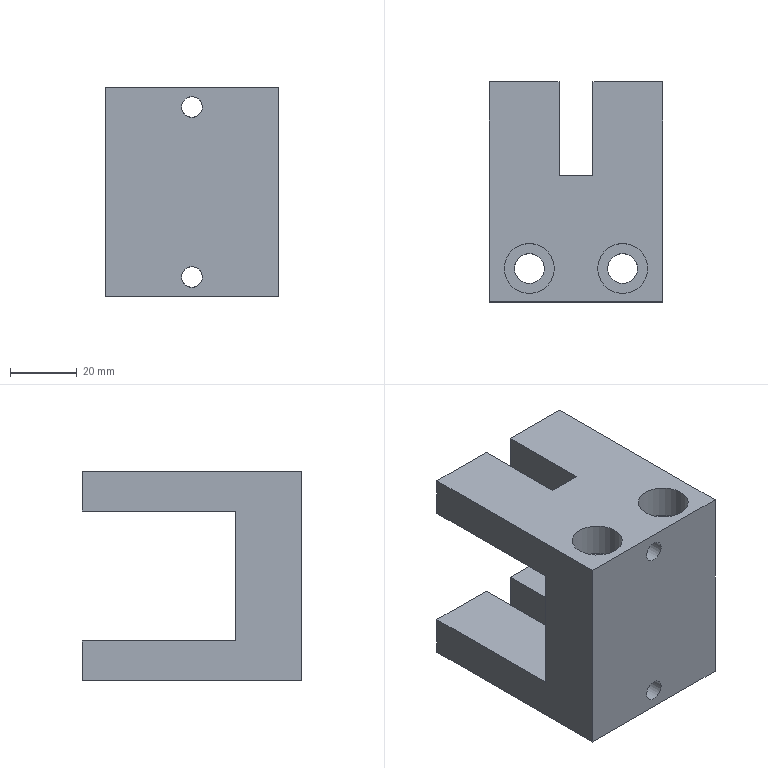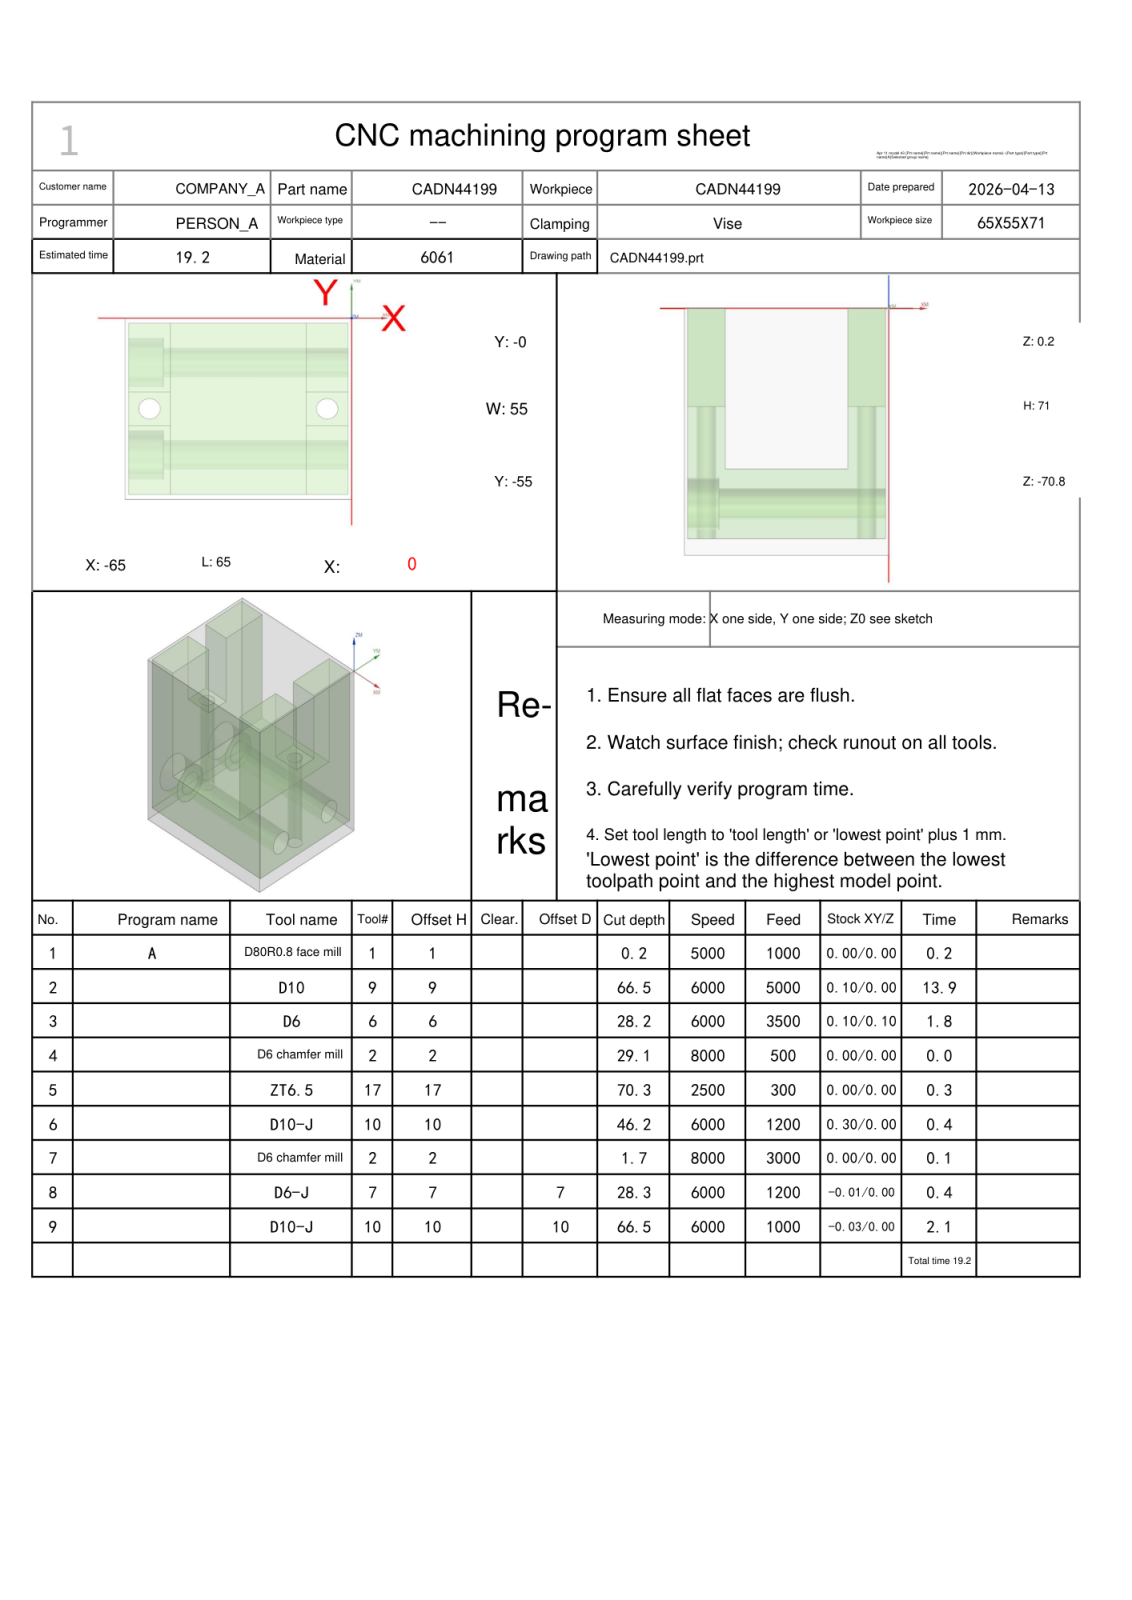NC program | NX | posted by the shop | part box 52 x 66 x 63 mm
Lines 3031 to 5259 of 5259:
N3 T06 M06
(D6  D=6. R=0. H=06 ce=0.10 di=0.10)
G00 G90 G54 X-70.1 Y-27.5 M03 S6000
G43 H06 Z20.
M08
Z.1
G01 Z-.4 F3500.
X-64.6
Y-29.5
X-51.4
Y-25.5
X-64.6
Y-27.5
Y-28.
Z.1
G00 Z.5
X-70.1 Y-27.5
Z-.3
G01 Z-.8
X-64.6
Y-29.5
X-51.4
Y-25.5
X-64.6
Y-27.5
Y-28.
Z-.3
G00 Z.1
X-70.1 Y-27.5
Z-.7
G01 Z-1.2
X-64.6
Y-29.5
X-51.4
Y-25.5
X-64.6
Y-27.5
Y-28.
Z-.7
G00 Z-.3
X-70.1 Y-27.5
Z-1.1
G01 Z-1.6
X-64.6
Y-29.5
X-51.4
Y-25.5
X-64.6
Y-27.5
Y-28.
Z-1.1
G00 Z-.7
X-70.1 Y-27.5
Z-1.5
G01 Z-2.
X-64.6
Y-29.5
X-51.4
Y-25.5
X-64.6
Y-27.5
Y-28.
Z-1.5
G00 Z-1.1
X-70.1 Y-27.5
Z-1.9
G01 Z-2.4
X-64.6
Y-29.5
X-51.4
Y-25.5
X-64.6
Y-27.5
Y-28.
Z-1.9
G00 Z-1.5
X-70.1 Y-27.5
Z-2.3
G01 Z-2.8
X-64.6
Y-29.5
X-51.4
Y-25.5
X-64.6
Y-27.5
Y-28.
Z-2.3
G00 Z-1.9
X-70.1 Y-27.5
Z-2.7
G01 Z-3.2
X-64.6
Y-29.5
X-51.4
Y-25.5
X-64.6
Y-27.5
Y-28.
Z-2.7
G00 Z-2.3
X-70.1 Y-27.5
Z-3.1
G01 Z-3.6
X-64.6
Y-29.5
X-51.4
Y-25.5
X-64.6
Y-27.5
Y-28.
Z-3.1
G00 Z-2.7
X-70.1 Y-27.5
Z-3.5
G01 Z-4.
X-64.6
Y-29.5
X-51.4
Y-25.5
X-64.6
Y-27.5
Y-28.
Z-3.5
G00 Z-3.1
X-70.1 Y-27.5
Z-3.9
G01 Z-4.4
X-64.6
Y-29.5
X-51.4
Y-25.5
X-64.6
Y-27.5
Y-28.
Z-3.9
G00 Z-3.5
X-70.1 Y-27.5
Z-4.3
G01 Z-4.8
X-64.6
Y-29.5
X-51.4
Y-25.5
X-64.6
Y-27.5
Y-28.
Z-4.3
G00 Z-3.9
X-70.1 Y-27.5
Z-4.7
G01 Z-5.2
X-64.6
Y-29.5
X-51.4
Y-25.5
X-64.6
Y-27.5
Y-28.
Z-4.7
G00 Z-4.3
X-70.1 Y-27.5
Z-5.1
G01 Z-5.6
X-64.6
Y-29.5
X-51.4
Y-25.5
X-64.6
Y-27.5
Y-28.
Z-5.1
G00 Z-4.7
X-70.1 Y-27.5
Z-5.5
G01 Z-6.
X-64.6
Y-29.5
X-51.4
Y-25.5
X-64.6
Y-27.5
Y-28.
Z-5.5
G00 Z-5.1
X-70.1 Y-27.5
Z-5.9
G01 Z-6.4
X-64.6
Y-29.5
X-51.4
Y-25.5
X-64.6
Y-27.5
Y-28.
Z-5.9
G00 Z-5.5
X-70.1 Y-27.5
Z-6.3
G01 Z-6.8
X-64.6
Y-29.5
X-51.4
Y-25.5
X-64.6
Y-27.5
Y-28.
Z-6.3
G00 Z-5.9
X-70.1 Y-27.5
Z-6.7
G01 Z-7.2
X-64.6
Y-29.5
X-51.4
Y-25.5
X-64.6
Y-27.5
Y-28.
Z-6.7
G00 Z-6.3
X-70.1 Y-27.5
Z-7.1
G01 Z-7.6
X-64.6
Y-29.5
X-51.4
Y-25.5
X-64.6
Y-27.5
Y-28.
Z-7.1
G00 Z-6.7
X-70.1 Y-27.5
Z-7.5
G01 Z-8.
X-64.6
Y-29.5
X-51.4
Y-25.5
X-64.6
Y-27.5
Y-28.
Z-7.5
G00 Z-7.1
X-70.1 Y-27.5
Z-7.9
G01 Z-8.4
X-64.6
Y-29.5
X-51.4
Y-25.5
X-64.6
Y-27.5
Y-28.
Z-7.9
G00 Z-7.5
X-70.1 Y-27.5
Z-8.3
G01 Z-8.8
X-64.6
Y-29.5
X-51.4
Y-25.5
X-64.6
Y-27.5
Y-28.
Z-8.3
G00 Z-7.9
X-70.1 Y-27.5
Z-8.7
G01 Z-9.2
X-64.6
Y-29.5
X-51.4
Y-25.5
X-64.6
Y-27.5
Y-28.
Z-8.7
G00 Z-8.3
X-70.1 Y-27.5
Z-9.1
G01 Z-9.6
X-64.6
Y-29.5
X-51.4
Y-25.5
X-64.6
Y-27.5
Y-28.
Z-9.1
G00 Z-8.7
X-70.1 Y-27.5
Z-9.5
G01 Z-10.
X-64.6
Y-29.5
X-51.4
Y-25.5
X-64.6
Y-27.5
Y-28.
Z-9.5
G00 Z-9.1
X-70.1 Y-27.5
Z-9.9
G01 Z-10.4
X-64.6
Y-29.5
X-51.4
Y-25.5
X-64.6
Y-27.5
Y-28.
Z-9.9
G00 Z-9.5
X-70.1 Y-27.5
Z-10.3
G01 Z-10.8
X-64.6
Y-29.5
X-51.4
Y-25.5
X-64.6
Y-27.5
Y-28.
Z-10.3
G00 Z-9.9
X-70.1 Y-27.5
Z-10.7
G01 Z-11.2
X-64.6
Y-29.5
X-51.4
Y-25.5
X-64.6
Y-27.5
Y-28.
Z-10.7
G00 Z-10.3
X-70.1 Y-27.5
Z-11.1
G01 Z-11.6
X-64.6
Y-29.5
X-51.4
Y-25.5
X-64.6
Y-27.5
Y-28.
Z-11.1
G00 Z-10.7
X-70.1 Y-27.5
Z-11.5
G01 Z-12.
X-64.6
Y-29.5
X-51.4
Y-25.5
X-64.6
Y-27.5
Y-28.
Z-11.5
G00 Z-11.1
X-70.1 Y-27.5
Z-11.9
G01 Z-12.4
X-64.6
Y-29.5
X-51.4
Y-25.5
X-64.6
Y-27.5
Y-28.
Z-11.9
G00 Z-11.5
X-70.1 Y-27.5
Z-12.3
G01 Z-12.8
X-64.6
Y-29.5
X-51.4
Y-25.5
X-64.6
Y-27.5
Y-28.
Z-12.3
G00 Z-11.9
X-70.1 Y-27.5
Z-12.7
G01 Z-13.2
X-64.6
Y-29.5
X-51.4
Y-25.5
X-64.6
Y-27.5
Y-28.
Z-12.7
G00 Z-12.3
X-70.1 Y-27.5
Z-13.1
G01 Z-13.6
X-64.6
Y-29.5
X-51.4
Y-25.5
X-64.6
Y-27.5
Y-28.
Z-13.1
G00 Z-12.7
X-70.1 Y-27.5
Z-13.5
G01 Z-14.
X-64.6
Y-29.5
X-51.4
Y-25.5
X-64.6
Y-27.5
Y-28.
Z-13.5
G00 Z-13.1
X-70.1 Y-27.5
Z-13.9
G01 Z-14.4
X-64.6
Y-29.5
X-51.4
Y-25.5
X-64.6
Y-27.5
Y-28.
Z-13.9
G00 Z-13.5
X-70.1 Y-27.5
Z-14.3
G01 Z-14.8
X-64.6
Y-29.5
X-51.4
Y-25.5
X-64.6
Y-27.5
Y-28.
Z-14.3
G00 Z-13.9
X-70.1 Y-27.5
Z-14.7
G01 Z-15.2
X-64.6
Y-29.5
X-51.4
Y-25.5
X-64.6
Y-27.5
Y-28.
Z-14.7
G00 Z-14.3
X-70.1 Y-27.5
Z-15.1
G01 Z-15.6
X-64.6
Y-29.5
X-51.4
Y-25.5
X-64.6
Y-27.5
Y-28.
Z-15.1
G00 Z-14.7
X-70.1 Y-27.5
Z-15.5
G01 Z-16.
X-64.6
Y-29.5
X-51.4
Y-25.5
X-64.6
Y-27.5
Y-28.
Z-15.5
G00 Z-15.1
X-70.1 Y-27.5
Z-15.9
G01 Z-16.4
X-64.6
Y-29.5
X-51.4
Y-25.5
X-64.6
Y-27.5
Y-28.
Z-15.9
G00 Z-15.5
X-70.1 Y-27.5
Z-16.3
G01 Z-16.8
X-64.6
Y-29.5
X-51.4
Y-25.5
X-64.6
Y-27.5
Y-28.
Z-16.3
G00 Z-15.9
X-70.1 Y-27.5
Z-16.7
G01 Z-17.2
X-64.6
Y-29.5
X-51.4
Y-25.5
X-64.6
Y-27.5
Y-28.
Z-16.7
G00 Z-16.3
X-70.1 Y-27.5
Z-17.1
G01 Z-17.6
X-64.6
Y-29.5
X-51.4
Y-25.5
X-64.6
Y-27.5
Y-28.
Z-17.1
G00 Z-16.7
X-70.1 Y-27.5
Z-17.5
G01 Z-18.
X-64.6
Y-29.5
X-51.4
Y-25.5
X-64.6
Y-27.5
Y-28.
Z-17.5
G00 Z-17.1
X-70.1 Y-27.5
Z-17.9
G01 Z-18.4
X-64.6
Y-29.5
X-51.4
Y-25.5
X-64.6
Y-27.5
Y-28.
Z-17.9
G00 Z-17.5
X-70.1 Y-27.5
Z-18.3
G01 Z-18.8
X-64.6
Y-29.5
X-51.4
Y-25.5
X-64.6
Y-27.5
Y-28.
Z-18.3
G00 Z-17.9
X-70.1 Y-27.5
Z-18.7
G01 Z-19.2
X-64.6
Y-29.5
X-51.4
Y-25.5
X-64.6
Y-27.5
Y-28.
Z-18.7
G00 Z-18.3
X-70.1 Y-27.5
Z-19.1
G01 Z-19.6
X-64.6
Y-29.5
X-51.4
Y-25.5
X-64.6
Y-27.5
Y-28.
Z-19.1
G00 Z-18.7
X-70.1 Y-27.5
Z-19.5
G01 Z-20.
X-64.6
Y-29.5
X-51.4
Y-25.5
X-64.6
Y-27.5
Y-28.
Z-19.5
G00 Z-19.1
X-70.1 Y-27.5
Z-19.9
G01 Z-20.4
X-64.6
Y-29.5
X-51.4
Y-25.5
X-64.6
Y-27.5
Y-28.
Z-19.9
G00 Z-19.5
X-70.1 Y-27.5
Z-20.3
G01 Z-20.8
X-64.6
Y-29.5
X-51.4
Y-25.5
X-64.6
Y-27.5
Y-28.
Z-20.3
G00 Z-19.9
X-70.1 Y-27.5
Z-20.7
G01 Z-21.2
X-64.6
Y-29.5
X-51.4
Y-25.5
X-64.6
Y-27.5
Y-28.
Z-20.7
G00 Z-20.3
X-70.1 Y-27.5
Z-21.1
G01 Z-21.6
X-64.6
Y-29.5
X-51.4
Y-25.5
X-64.6
Y-27.5
Y-28.
Z-21.1
G00 Z-20.7
X-70.1 Y-27.5
Z-21.5
G01 Z-22.
X-64.6
Y-29.5
X-51.4
Y-25.5
X-64.6
Y-27.5
Y-28.
Z-21.5
G00 Z-21.1
X-70.1 Y-27.5
Z-21.9
G01 Z-22.4
X-64.6
Y-29.5
X-51.4
Y-25.5
X-64.6
Y-27.5
Y-28.
Z-21.9
G00 Z-21.5
X-70.1 Y-27.5
Z-22.3
G01 Z-22.8
X-64.6
Y-29.5
X-51.4
Y-25.5
X-64.6
Y-27.5
Y-28.
Z-22.3
G00 Z-21.9
X-70.1 Y-27.5
Z-22.7
G01 Z-23.2
X-64.6
Y-29.5
X-51.4
Y-25.5
X-64.6
Y-27.5
Y-28.
Z-22.7
G00 Z-22.3
X-70.1 Y-27.5
Z-23.1
G01 Z-23.6
X-64.6
Y-29.5
X-51.4
Y-25.5
X-64.6
Y-27.5
Y-28.
Z-23.1
G00 Z-22.7
X-70.1 Y-27.5
Z-23.5
G01 Z-24.
X-64.6
Y-29.5
X-51.4
Y-25.5
X-64.6
Y-27.5
Y-28.
Z-23.5
G00 Z-23.1
X-70.1 Y-27.5
Z-23.9
G01 Z-24.4
X-64.6
Y-29.5
X-51.4
Y-25.5
X-64.6
Y-27.5
Y-28.
Z-23.9
G00 Z-23.5
X-70.1 Y-27.5
Z-24.3
G01 Z-24.8
X-64.6
Y-29.5
X-51.4
Y-25.5
X-64.6
Y-27.5
Y-28.
Z-24.3
G00 Z-23.9
X-70.1 Y-27.5
Z-24.7
G01 Z-25.2
X-64.6
Y-29.5
X-51.4
Y-25.5
X-64.6
Y-27.5
Y-28.
Z-24.7
G00 Z-24.3
X-70.1 Y-27.5
Z-25.1
G01 Z-25.6
X-64.6
Y-29.5
X-51.4
Y-25.5
X-64.6
Y-27.5
Y-28.
Z-25.1
G00 Z-24.7
X-70.1 Y-27.5
Z-25.5
G01 Z-26.
X-64.6
Y-29.5
X-51.4
Y-25.5
X-64.6
Y-27.5
Y-28.
Z-25.5
G00 Z-25.1
X-70.1 Y-27.5
Z-25.9
G01 Z-26.4
X-64.6
Y-29.5
X-51.4
Y-25.5
X-64.6
Y-27.5
Y-28.
Z-25.9
G00 Z-25.5
X-70.1 Y-27.5
Z-26.3
G01 Z-26.8
X-64.6
Y-29.5
X-51.4
Y-25.5
X-64.6
Y-27.5
Y-28.
Z-26.3
G00 Z-25.9
X-70.1 Y-27.5
Z-26.7
G01 Z-27.2
X-64.6
Y-29.5
X-51.4
Y-25.5
X-64.6
Y-27.5
Y-28.
Z-26.7
G00 Z-26.3
X-70.1 Y-27.5
Z-27.1
G01 Z-27.6
X-64.6
Y-29.5
X-51.4
Y-25.5
X-64.6
Y-27.5
Y-28.
Z-27.1
G00 Z-26.7
X-70.1 Y-27.5
Z-27.5
G01 Z-28.
X-64.6
Y-29.5
X-51.4
Y-25.5
X-64.6
Y-27.5
Y-28.
Z-27.5
G00 Z20.
X5.1 Y-27.5
Z.1
G01 Z-.4
X-.4
Y-25.5
X-13.6
Y-29.5
X-.4
Y-27.5
Y-27.
Z.1
G00 Z.5
X5.1 Y-27.5
Z-.3
G01 Z-.8
X-.4
Y-25.5
X-13.6
Y-29.5
X-.4
Y-27.5
Y-27.
Z-.3
G00 Z.1
X5.1 Y-27.5
Z-.7
G01 Z-1.2
X-.4
Y-25.5
X-13.6
Y-29.5
X-.4
Y-27.5
Y-27.
Z-.7
G00 Z-.3
X5.1 Y-27.5
Z-1.1
G01 Z-1.6
X-.4
Y-25.5
X-13.6
Y-29.5
X-.4
Y-27.5
Y-27.
Z-1.1
G00 Z-.7
X5.1 Y-27.5
Z-1.5
G01 Z-2.
X-.4
Y-25.5
X-13.6
Y-29.5
X-.4
Y-27.5
Y-27.
Z-1.5
G00 Z-1.1
X5.1 Y-27.5
Z-1.9
G01 Z-2.4
X-.4
Y-25.5
X-13.6
Y-29.5
X-.4
Y-27.5
Y-27.
Z-1.9
G00 Z-1.5
X5.1 Y-27.5
Z-2.3
G01 Z-2.8
X-.4
Y-25.5
X-13.6
Y-29.5
X-.4
Y-27.5
Y-27.
Z-2.3
G00 Z-1.9
X5.1 Y-27.5
Z-2.7
G01 Z-3.2
X-.4
Y-25.5
X-13.6
Y-29.5
X-.4
Y-27.5
Y-27.
Z-2.7
G00 Z-2.3
X5.1 Y-27.5
Z-3.1
G01 Z-3.6
X-.4
Y-25.5
X-13.6
Y-29.5
X-.4
Y-27.5
Y-27.
Z-3.1
G00 Z-2.7
X5.1 Y-27.5
Z-3.5
G01 Z-4.
X-.4
Y-25.5
X-13.6
Y-29.5
X-.4
Y-27.5
Y-27.
Z-3.5
G00 Z-3.1
X5.1 Y-27.5
Z-3.9
G01 Z-4.4
X-.4
Y-25.5
X-13.6
Y-29.5
X-.4
Y-27.5
Y-27.
Z-3.9
G00 Z-3.5
X5.1 Y-27.5
Z-4.3
G01 Z-4.8
X-.4
Y-25.5
X-13.6
Y-29.5
X-.4
Y-27.5
Y-27.
Z-4.3
G00 Z-3.9
X5.1 Y-27.5
Z-4.7
G01 Z-5.2
X-.4
Y-25.5
X-13.6
Y-29.5
X-.4
Y-27.5
Y-27.
Z-4.7
G00 Z-4.3
X5.1 Y-27.5
Z-5.1
G01 Z-5.6
X-.4
Y-25.5
X-13.6
Y-29.5
X-.4
Y-27.5
Y-27.
Z-5.1
G00 Z-4.7
X5.1 Y-27.5
Z-5.5
G01 Z-6.
X-.4
Y-25.5
X-13.6
Y-29.5
X-.4
Y-27.5
Y-27.
Z-5.5
G00 Z-5.1
X5.1 Y-27.5
Z-5.9
G01 Z-6.4
X-.4
Y-25.5
X-13.6
Y-29.5
X-.4
Y-27.5
Y-27.
Z-5.9
G00 Z-5.5
X5.1 Y-27.5
Z-6.3
G01 Z-6.8
X-.4
Y-25.5
X-13.6
Y-29.5
X-.4
Y-27.5
Y-27.
Z-6.3
G00 Z-5.9
X5.1 Y-27.5
Z-6.7
G01 Z-7.2
X-.4
Y-25.5
X-13.6
Y-29.5
X-.4
Y-27.5
Y-27.
Z-6.7
G00 Z-6.3
X5.1 Y-27.5
Z-7.1
G01 Z-7.6
X-.4
Y-25.5
X-13.6
Y-29.5
X-.4
Y-27.5
Y-27.
Z-7.1
G00 Z-6.7
X5.1 Y-27.5
Z-7.5
G01 Z-8.
X-.4
Y-25.5
X-13.6
Y-29.5
X-.4
Y-27.5
Y-27.
Z-7.5
G00 Z-7.1
X5.1 Y-27.5
Z-7.9
G01 Z-8.4
X-.4
Y-25.5
X-13.6
Y-29.5
X-.4
Y-27.5
Y-27.
Z-7.9
G00 Z-7.5
X5.1 Y-27.5
Z-8.3
G01 Z-8.8
X-.4
Y-25.5
X-13.6
Y-29.5
X-.4
Y-27.5
Y-27.
Z-8.3
G00 Z-7.9
X5.1 Y-27.5
Z-8.7
G01 Z-9.2
X-.4
Y-25.5
X-13.6
Y-29.5
X-.4
Y-27.5
Y-27.
Z-8.7
G00 Z-8.3
X5.1 Y-27.5
Z-9.1
G01 Z-9.6
X-.4
Y-25.5
X-13.6
Y-29.5
X-.4
Y-27.5
Y-27.
Z-9.1
G00 Z-8.7
X5.1 Y-27.5
Z-9.5
G01 Z-10.
X-.4
Y-25.5
X-13.6
Y-29.5
X-.4
Y-27.5
Y-27.
Z-9.5
G00 Z-9.1
X5.1 Y-27.5
Z-9.9
G01 Z-10.4
X-.4
Y-25.5
X-13.6
Y-29.5
X-.4
Y-27.5
Y-27.
Z-9.9
G00 Z-9.5
X5.1 Y-27.5
Z-10.3
G01 Z-10.8
X-.4
Y-25.5
X-13.6
Y-29.5
X-.4
Y-27.5
Y-27.
Z-10.3
G00 Z-9.9
X5.1 Y-27.5
Z-10.7
G01 Z-11.2
X-.4
Y-25.5
X-13.6
Y-29.5
X-.4
Y-27.5
Y-27.
Z-10.7
G00 Z-10.3
X5.1 Y-27.5
Z-11.1
G01 Z-11.6
X-.4
Y-25.5
X-13.6
Y-29.5
X-.4
Y-27.5
Y-27.
Z-11.1
G00 Z-10.7
X5.1 Y-27.5
Z-11.5
G01 Z-12.
X-.4
Y-25.5
X-13.6
Y-29.5
X-.4
Y-27.5
Y-27.
Z-11.5
G00 Z-11.1
X5.1 Y-27.5
Z-11.9
G01 Z-12.4
X-.4
Y-25.5
X-13.6
Y-29.5
X-.4
Y-27.5
Y-27.
Z-11.9
G00 Z-11.5
X5.1 Y-27.5
Z-12.3
G01 Z-12.8
X-.4
Y-25.5
X-13.6
Y-29.5
X-.4
Y-27.5
Y-27.
Z-12.3
G00 Z-11.9
X5.1 Y-27.5
Z-12.7
G01 Z-13.2
X-.4
Y-25.5
X-13.6
Y-29.5
X-.4
Y-27.5
Y-27.
Z-12.7
G00 Z-12.3
X5.1 Y-27.5
Z-13.1
G01 Z-13.6
X-.4
Y-25.5
X-13.6
Y-29.5
X-.4
Y-27.5
Y-27.
Z-13.1
G00 Z-12.7
X5.1 Y-27.5
Z-13.5
G01 Z-14.
X-.4
Y-25.5
X-13.6
Y-29.5
X-.4
Y-27.5
Y-27.
Z-13.5
G00 Z-13.1
X5.1 Y-27.5
Z-13.9
G01 Z-14.4
X-.4
Y-25.5
X-13.6
Y-29.5
X-.4
Y-27.5
Y-27.
Z-13.9
G00 Z-13.5
X5.1 Y-27.5
Z-14.3
G01 Z-14.8
X-.4
Y-25.5
X-13.6
Y-29.5
X-.4
Y-27.5
Y-27.
Z-14.3
G00 Z-13.9
X5.1 Y-27.5
Z-14.7
G01 Z-15.2
X-.4
Y-25.5
X-13.6
Y-29.5
X-.4
Y-27.5
Y-27.
Z-14.7
G00 Z-14.3
X5.1 Y-27.5
Z-15.1
G01 Z-15.6
X-.4
Y-25.5
X-13.6
Y-29.5
X-.4
Y-27.5
Y-27.
Z-15.1
G00 Z-14.7
X5.1 Y-27.5
Z-15.5
G01 Z-16.
X-.4
Y-25.5
X-13.6
Y-29.5
X-.4
Y-27.5
Y-27.
Z-15.5
G00 Z-15.1
X5.1 Y-27.5
Z-15.9
G01 Z-16.4
X-.4
Y-25.5
X-13.6
Y-29.5
X-.4
Y-27.5
Y-27.
Z-15.9
G00 Z-15.5
X5.1 Y-27.5
Z-16.3
G01 Z-16.8
X-.4
Y-25.5
X-13.6
Y-29.5
X-.4
Y-27.5
Y-27.
Z-16.3
G00 Z-15.9
X5.1 Y-27.5
Z-16.7
G01 Z-17.2
X-.4
Y-25.5
X-13.6
Y-29.5
X-.4
Y-27.5
Y-27.
Z-16.7
G00 Z-16.3
X5.1 Y-27.5
Z-17.1
G01 Z-17.6
X-.4
Y-25.5
X-13.6
Y-29.5
X-.4
Y-27.5
Y-27.
Z-17.1
G00 Z-16.7
X5.1 Y-27.5
Z-17.5
G01 Z-18.
X-.4
Y-25.5
X-13.6
Y-29.5
X-.4
Y-27.5
Y-27.
Z-17.5
G00 Z-17.1
X5.1 Y-27.5
Z-17.9
G01 Z-18.4
X-.4
Y-25.5
X-13.6
Y-29.5
X-.4
Y-27.5
Y-27.
Z-17.9
G00 Z-17.5
X5.1 Y-27.5
Z-18.3
G01 Z-18.8
X-.4
Y-25.5
X-13.6
Y-29.5
X-.4
Y-27.5
Y-27.
Z-18.3
G00 Z-17.9
X5.1 Y-27.5
Z-18.7
G01 Z-19.2
X-.4
Y-25.5
X-13.6
Y-29.5
X-.4
Y-27.5
Y-27.
Z-18.7
G00 Z-18.3
X5.1 Y-27.5
Z-19.1
G01 Z-19.6
X-.4
Y-25.5
X-13.6
Y-29.5
X-.4
Y-27.5
Y-27.
Z-19.1
G00 Z-18.7
X5.1 Y-27.5
Z-19.5
G01 Z-20.
X-.4
Y-25.5
X-13.6
Y-29.5
X-.4
Y-27.5
Y-27.
Z-19.5
G00 Z-19.1
X5.1 Y-27.5
Z-19.9
G01 Z-20.4
X-.4
Y-25.5
X-13.6
Y-29.5
X-.4
Y-27.5
Y-27.
Z-19.9
G00 Z-19.5
X5.1 Y-27.5
Z-20.3
G01 Z-20.8
X-.4
Y-25.5
X-13.6
Y-29.5
X-.4
Y-27.5
Y-27.
Z-20.3
G00 Z-19.9
X5.1 Y-27.5
Z-20.7
G01 Z-21.2
X-.4
Y-25.5
X-13.6
Y-29.5
X-.4
Y-27.5
Y-27.
Z-20.7
G00 Z-20.3
X5.1 Y-27.5
Z-21.1
G01 Z-21.6
X-.4
Y-25.5
X-13.6
Y-29.5
X-.4
Y-27.5
Y-27.
Z-21.1
G00 Z-20.7
X5.1 Y-27.5
Z-21.5
G01 Z-22.
X-.4
Y-25.5
X-13.6
Y-29.5
X-.4
Y-27.5
Y-27.
Z-21.5
G00 Z-21.1
X5.1 Y-27.5
Z-21.9
G01 Z-22.4
X-.4
Y-25.5
X-13.6
Y-29.5
X-.4
Y-27.5
Y-27.
Z-21.9
G00 Z-21.5
X5.1 Y-27.5
Z-22.3
G01 Z-22.8
X-.4
Y-25.5
X-13.6
Y-29.5
X-.4
Y-27.5
Y-27.
Z-22.3
G00 Z-21.9
X5.1 Y-27.5
Z-22.7
G01 Z-23.2
X-.4
Y-25.5
X-13.6
Y-29.5
X-.4
Y-27.5
Y-27.
Z-22.7
G00 Z-22.3
X5.1 Y-27.5
Z-23.1
G01 Z-23.6
X-.4
Y-25.5
X-13.6
Y-29.5
X-.4
Y-27.5
Y-27.
Z-23.1
G00 Z-22.7
X5.1 Y-27.5
Z-23.5
G01 Z-24.
X-.4
Y-25.5
X-13.6
Y-29.5
X-.4
Y-27.5
Y-27.
Z-23.5
G00 Z-23.1
X5.1 Y-27.5
Z-23.9
G01 Z-24.4
X-.4
Y-25.5
X-13.6
Y-29.5
X-.4
Y-27.5
Y-27.
Z-23.9
G00 Z-23.5
X5.1 Y-27.5
Z-24.3
G01 Z-24.8
X-.4
Y-25.5
X-13.6
Y-29.5
X-.4
Y-27.5
Y-27.
Z-24.3
G00 Z-23.9
X5.1 Y-27.5
Z-24.7
G01 Z-25.2
X-.4
Y-25.5
X-13.6
Y-29.5
X-.4
Y-27.5
Y-27.
Z-24.7
G00 Z-24.3
X5.1 Y-27.5
Z-25.1
G01 Z-25.6
X-.4
Y-25.5
X-13.6
Y-29.5
X-.4
Y-27.5
Y-27.
Z-25.1
G00 Z-24.7
X5.1 Y-27.5
Z-25.5
G01 Z-26.
X-.4
Y-25.5
X-13.6
Y-29.5
X-.4
Y-27.5
Y-27.
Z-25.5
G00 Z-25.1
X5.1 Y-27.5
Z-25.9
G01 Z-26.4
X-.4
Y-25.5
X-13.6
Y-29.5
X-.4
Y-27.5
Y-27.
Z-25.9
G00 Z-25.5
X5.1 Y-27.5
Z-26.3
G01 Z-26.8
X-.4
Y-25.5
X-13.6
Y-29.5
X-.4
Y-27.5
Y-27.
Z-26.3
G00 Z-25.9
X5.1 Y-27.5
Z-26.7
G01 Z-27.2
X-.4
Y-25.5
X-13.6
Y-29.5
X-.4
Y-27.5
Y-27.
Z-26.7
G00 Z-26.3
X5.1 Y-27.5
Z-27.1
G01 Z-27.6
X-.4
Y-25.5
X-13.6
Y-29.5
X-.4
Y-27.5
Y-27.
Z-27.1
G00 Z-26.7
X5.1 Y-27.5
Z-27.5
G01 Z-28.
X-.4
Y-25.5
X-13.6
Y-29.5
X-.4
Y-27.5
Y-27.
Z-27.5
G00 Z20.
G91 G28 Z0.0
M05
M09
G91 G28 Z0.0
M01
N4 T02 M06
(D6 chamfer mill  D=6. R=0. H=02 ce=0.00 di=0.10)
G00 G90 G54 X-7. Y-27.5 M03 S8000
G43 H02 Z20.
M08
G98 G81 X-7. Y-27.5 Z-28.9 R-27.1 F500.
X-58.
G80
G00 Z20.
G91 G28 Z0.0
M05
M09
G91 G28 Z0.0
M01
N5 T17 M06
(ZT6.5 D=6.5 DR_a=118 H=17)
G00 G90 G54 X-7. Y-27.5 M03 S2500
G43 H17 Z20.
M08
G98 G83 X-7. Y-27.5 Z-70.1 R-27.1 F300. Q3.
X-58.
G80
G00 Z20.
G91 G28 Z0.0
M05
M09
G91 G28 Z0.0
M01
N6 T10 M06
(D10-J  D=10. R=0. H=10 ce=0.30 di=0.00)
G00 G90 G54 X-46.699 Y-61.8 M03 S6000
G43 H10 Z20.
M08
Z-45.5
G01 Z-46. F1200.
Y-58.5
Y3.5
X-41.019
Y-58.5
X-35.339
Y3.5
X-29.66
Y-58.5
X-23.98
Y3.5
X-18.3
Y-58.5
Y-61.8
Z-45.5
G00 Z20.
G91 G28 Z0.0
M05
M09
G91 G28 Z0.0
M01
N7 T02 M06
(D6 chamfer mill  D=6. R=0. H=02 ce=0.00 di=0.00)
G00 G90 G54 X-66.128 Y-12.2 M03 S8000
G43 H02 Z20.
M08
Z2.099
G01 Z-1.499 F3000.
G03 X-65.828 Y-12.28 I.3 J.52
X-65.308 Y-11.98 I0.0 J.6
G01 X-65.3 Y-11.95
Y-1.5
G02 X-64. Y-.2 I1.3 J0.0
G01 X-52.
G02 X-50.7 Y-1.5 I0.0 J-1.3
G01 Y-22.4
G02 X-52. Y-23.7 I-1.3 J0.0
G01 X-64.
G02 X-65.3 Y-22.4 I0.0 J1.3
G01 Y-11.95
X-65.308 Y-11.92
G03 X-65.828 Y-11.62 I-.52 J-.3
X-66.128 Y-11.7 I0.0 J-.6
G01 Z2.099
G00 Z20.
X-49.872 Y-42.8
Z2.099
G01 Z-1.499
G03 X-50.172 Y-42.72 I-.3 J-.52
X-50.692 Y-43.02 I0.0 J-.6
G01 X-50.7 Y-43.05
Y-53.5
G02 X-52. Y-54.8 I-1.3 J0.0
G01 X-64.
G02 X-65.3 Y-53.5 I0.0 J1.3
G01 Y-32.6
G02 X-64. Y-31.3 I1.3 J0.0
G01 X-52.
G02 X-50.7 Y-32.6 I0.0 J-1.3
G01 Y-43.05
X-50.692 Y-43.08
G03 X-50.172 Y-43.38 I.52 J.3
X-49.872 Y-43.3 I0.0 J.6
G01 Z2.099
G00 Z20.
X1.128 Y-42.8
Z2.099
G01 Z-1.499
G03 X.828 Y-42.72 I-.3 J-.52
X.308 Y-43.02 I0.0 J-.6
G01 X.3 Y-43.05
Y-53.5
G02 X-1. Y-54.8 I-1.3 J0.0
G01 X-13.
G02 X-14.3 Y-53.5 I0.0 J1.3
G01 Y-32.6
G02 X-13. Y-31.3 I1.3 J0.0
G01 X-1.
G02 X.3 Y-32.6 I0.0 J-1.3
G01 Y-43.05
X.308 Y-43.08
G03 X.828 Y-43.38 I.52 J.3
X1.128 Y-43.3 I0.0 J.6
G01 Z2.099
G00 Z20.
Y-11.7
Z2.099
G01 Z-1.499
G03 X.828 Y-11.62 I-.3 J-.52
X.308 Y-11.92 I0.0 J-.6
G01 X.3 Y-11.95
Y-22.4
G02 X-1. Y-23.7 I-1.3 J0.0
G01 X-13.
G02 X-14.3 Y-22.4 I0.0 J1.3
G01 Y-1.5
G02 X-13. Y-.2 I1.3 J0.0
G01 X-1.
G02 X.3 Y-1.5 I0.0 J-1.3
G01 Y-11.95
X.308 Y-11.98
G03 X.828 Y-12.28 I.52 J.3
X1.128 Y-12.2 I0.0 J.6
G01 Z2.099
G00 Z20.
G91 G28 Z0.0
M05
M09
G91 G28 Z0.0
M01
N8 T07 M06
(D6-J  D=6. R=0. H=07 ce=-0.01 di=0.00)
G00 G90 G54 X-67.7 Y-28.51 M03 S6000
G43 H07 Z20.
M08
Z-6.525
G01 Z-7.025 F1200.
G41 D07
Y-28.61
G03 X-66.7 Y-29.61 I1. J0.0
G01 X-49.3
G03 X-48.3 Y-28.61 I0.0 J1.
G01 G40 Y-28.51
Z-6.525
G00 Z20.
X-67.7
Z-13.55
G01 Z-14.05
G41 D07
Y-28.61
G03 X-66.7 Y-29.61 I1. J0.0
G01 X-49.3
G03 X-48.3 Y-28.61 I0.0 J1.
G01 G40 Y-28.51
Z-13.55
G00 Z20.
X-67.7
Z-20.575
G01 Z-21.075
G41 D07
Y-28.61
G03 X-66.7 Y-29.61 I1. J0.0
G01 X-49.3
G03 X-48.3 Y-28.61 I0.0 J1.
G01 G40 Y-28.51
Z-20.575
G00 Z20.
Y-26.49
Z-6.525
G01 Z-7.025
G41 D07
Y-26.39
G03 X-49.3 Y-25.39 I-1. J0.0
G01 X-66.7
G03 X-67.7 Y-26.39 I0.0 J-1.
G01 G40 Y-26.49
Z-6.525
G00 Z20.
X-48.3
Z-13.55
G01 Z-14.05
G41 D07
Y-26.39
G03 X-49.3 Y-25.39 I-1. J0.0
G01 X-66.7
G03 X-67.7 Y-26.39 I0.0 J-1.
G01 G40 Y-26.49
Z-13.55
G00 Z20.
X-48.3
Z-20.575
G01 Z-21.075
G41 D07
Y-26.39
G03 X-49.3 Y-25.39 I-1. J0.0
G01 X-66.7
G03 X-67.7 Y-26.39 I0.0 J-1.
G01 G40 Y-26.49
Z-20.575
G00 Z20.
Y-28.51
Z-27.6
G01 Z-28.1
G41 D07
Y-28.61
G03 X-66.7 Y-29.61 I1. J0.0
G01 X-49.3
G03 X-48.3 Y-28.61 I0.0 J1.
G01 G40 Y-28.51
Y-26.49
G41 D07
Y-26.39
G03 X-49.3 Y-25.39 I-1. J0.0
G01 X-66.7
G03 X-67.7 Y-26.39 I0.0 J-1.
G01 G40 Y-26.49
Z-27.6
G00 Z20.
X-16.7 Y-28.51
Z-6.525
G01 Z-7.025
G41 D07
Y-28.61
G03 X-15.7 Y-29.61 I1. J0.0
G01 X1.7
G03 X2.7 Y-28.61 I0.0 J1.
G01 G40 Y-28.51
Z-6.525
G00 Z20.
X-16.7
Z-13.55
G01 Z-14.05
G41 D07
Y-28.61
G03 X-15.7 Y-29.61 I1. J0.0
G01 X1.7
G03 X2.7 Y-28.61 I0.0 J1.
G01 G40 Y-28.51
Z-13.55
G00 Z20.
X-16.7
Z-20.575
G01 Z-21.075
G41 D07
Y-28.61
G03 X-15.7 Y-29.61 I1. J0.0
G01 X1.7
G03 X2.7 Y-28.61 I0.0 J1.
G01 G40 Y-28.51
Z-20.575
G00 Z20.
Y-26.49
Z-6.525
G01 Z-7.025
G41 D07
Y-26.39
G03 X1.7 Y-25.39 I-1. J0.0
G01 X-15.7
G03 X-16.7 Y-26.39 I0.0 J-1.
G01 G40 Y-26.49
Z-6.525
G00 Z20.
X2.7
Z-13.55
G01 Z-14.05
G41 D07
Y-26.39
G03 X1.7 Y-25.39 I-1. J0.0
G01 X-15.7
G03 X-16.7 Y-26.39 I0.0 J-1.
G01 G40 Y-26.49
Z-13.55
G00 Z20.
X2.7
Z-20.575
G01 Z-21.075
G41 D07
Y-26.39
G03 X1.7 Y-25.39 I-1. J0.0
G01 X-15.7
G03 X-16.7 Y-26.39 I0.0 J-1.
G01 G40 Y-26.49
Z-20.575
G00 Z20.
Y-28.51
Z-27.6
G01 Z-28.1
G41 D07
Y-28.61
G03 X-15.7 Y-29.61 I1. J0.0
G01 X1.7
G03 X2.7 Y-28.61 I0.0 J1.
G01 G40 Y-28.51
Y-26.49
G41 D07
Y-26.39
G03 X1.7 Y-25.39 I-1. J0.0
G01 X-15.7
G03 X-16.7 Y-26.39 I0.0 J-1.
G01 G40 Y-26.49
Z-27.6
G00 Z20.
G91 G28 Z0.0
M05
M09
G91 G28 Z0.0
M01
N9 T10 M06
(D10-J  D=10. R=0. H=10 ce=-0.03 di=0.01)
G00 G90 G54 X-45.925 Y4. M03 S6000
G43 H10 Z20.
M08
Z-7.166
G01 Z-7.666 F1000.
G41 D10
X-46.025
G03 X-47.025 Y3. I0.0 J-1.
G01 Y-58.
G03 X-46.025 Y-59. I1. J0.0
G01 G40 X-45.925
Z-7.166
G00 Z20.
Y4.
Z-14.832
G01 Z-15.332
G41 D10
X-46.025
G03 X-47.025 Y3. I0.0 J-1.
G01 Y-58.
G03 X-46.025 Y-59. I1. J0.0
G01 G40 X-45.925
Z-14.832
G00 Z20.
Y4.
Z-22.498
G01 Z-22.998
G41 D10
X-46.025
G03 X-47.025 Y3. I0.0 J-1.
G01 Y-58.
G03 X-46.025 Y-59. I1. J0.0
G01 G40 X-45.925
Z-22.498
G00 Z20.
Y4.
Z-30.163
G01 Z-30.663
G41 D10
X-46.025
G03 X-47.025 Y3. I0.0 J-1.
G01 Y-58.
G03 X-46.025 Y-59. I1. J0.0
G01 G40 X-45.925
Z-30.163
G00 Z20.
Y4.
Z-37.829
G01 Z-38.329
G41 D10
X-46.025
G03 X-47.025 Y3. I0.0 J-1.
G01 Y-58.
G03 X-46.025 Y-59. I1. J0.0
G01 G40 X-45.925
Z-37.829
G00 Z20.
X-19.075
Z-7.166
G01 Z-7.666
G41 D10
X-18.975
G03 X-17.975 Y-58. I0.0 J1.
G01 Y3.
G03 X-18.975 Y4. I-1. J0.0
G01 G40 X-19.075
Z-7.166
G00 Z20.
Y-59.
Z-14.832
G01 Z-15.332
G41 D10
X-18.975
G03 X-17.975 Y-58. I0.0 J1.
G01 Y3.
G03 X-18.975 Y4. I-1. J0.0
G01 G40 X-19.075
Z-14.832
G00 Z20.
Y-59.
Z-22.498
G01 Z-22.998
G41 D10
X-18.975
G03 X-17.975 Y-58. I0.0 J1.
G01 Y3.
G03 X-18.975 Y4. I-1. J0.0
G01 G40 X-19.075
Z-22.498
G00 Z20.
Y-59.
Z-30.163
G01 Z-30.663
G41 D10
X-18.975
G03 X-17.975 Y-58. I0.0 J1.
G01 Y3.
G03 X-18.975 Y4. I-1. J0.0
G01 G40 X-19.075
Z-30.163
G00 Z20.
Y-59.
Z-37.829
G01 Z-38.329
G41 D10
X-18.975
G03 X-17.975 Y-58. I0.0 J1.
G01 Y3.
G03 X-18.975 Y4. I-1. J0.0
G01 G40 X-19.075
Z-37.829
G00 Z20.
X-45.925
Z-45.495
G01 Z-45.995
G41 D10
X-46.025
G03 X-47.025 Y3. I0.0 J-1.
G01 Y-58.
G03 X-46.025 Y-59. I1. J0.0
G01 G40 X-45.925
Z-45.495
G00 Z20.
X-19.075
Z-45.495
G01 Z-45.995
G41 D10
X-18.975
G03 X-17.975 Y-58. I0.0 J1.
G01 Y3.
G03 X-18.975 Y4. I-1. J0.0
G01 G40 X-19.075
Z-45.495
G00 Z20.
G00 G90 X-65.013 Y4.616 M03 S6000
Z20.
Z-16.075
G01 Z-16.575 F1000.
G41 D10
X-64.997 Y4.417
G03 X-64. Y3.5 I.997 J.083
G01 X-1.
G02 X4. Y-1.5 I0.0 J-5.
G01 Y-53.5
G02 X-1. Y-58.5 I-5. J0.0
G01 X-64.
G02 X-69. Y-53.5 I0.0 J5.
G01 Y-1.5
G02 X-64. Y3.5 I5. J0.0
G01 X-63.5
G03 X-62.5 Y4.5 I0.0 J1.
G01 G40 Y4.7
Z-16.075
G00 Z20.
X-65.013 Y4.616
Z-32.65
G01 Z-33.15
G41 D10
X-64.997 Y4.417
G03 X-64. Y3.5 I.997 J.083
G01 X-1.
G02 X4. Y-1.5 I0.0 J-5.
G01 Y-53.5
G02 X-1. Y-58.5 I-5. J0.0
G01 X-64.
G02 X-69. Y-53.5 I0.0 J5.
G01 Y-1.5
G02 X-64. Y3.5 I5. J0.0
G01 X-63.5
G03 X-62.5 Y4.5 I0.0 J1.
G01 G40 Y4.7
Z-32.65
G00 Z20.
X-65.013 Y4.616
Z-49.225
G01 Z-49.725
G41 D10
X-64.997 Y4.417
G03 X-64. Y3.5 I.997 J.083
G01 X-1.
G02 X4. Y-1.5 I0.0 J-5.
G01 Y-53.5
G02 X-1. Y-58.5 I-5. J0.0
G01 X-64.
G02 X-69. Y-53.5 I0.0 J5.
G01 Y-1.5
G02 X-64. Y3.5 I5. J0.0
G01 X-63.5
G03 X-62.5 Y4.5 I0.0 J1.
G01 G40 Y4.7
Z-49.225
G00 Z20.
X-65.013 Y4.616
Z-65.8
G01 Z-66.3
G41 D10
X-64.997 Y4.417
G03 X-64. Y3.5 I.997 J.083
G01 X-1.
G02 X4. Y-1.5 I0.0 J-5.
G01 Y-53.5
G02 X-1. Y-58.5 I-5. J0.0
G01 X-64.
G02 X-69. Y-53.5 I0.0 J5.
G01 Y-1.5
G02 X-64. Y3.5 I5. J0.0
G01 X-63.5
G03 X-62.5 Y4.5 I0.0 J1.
G01 G40 Y4.7
Z-65.8
G00 Z20.
M05
M09
G91 G28 Z0.0
G91 G28 Y0.0
M30
%